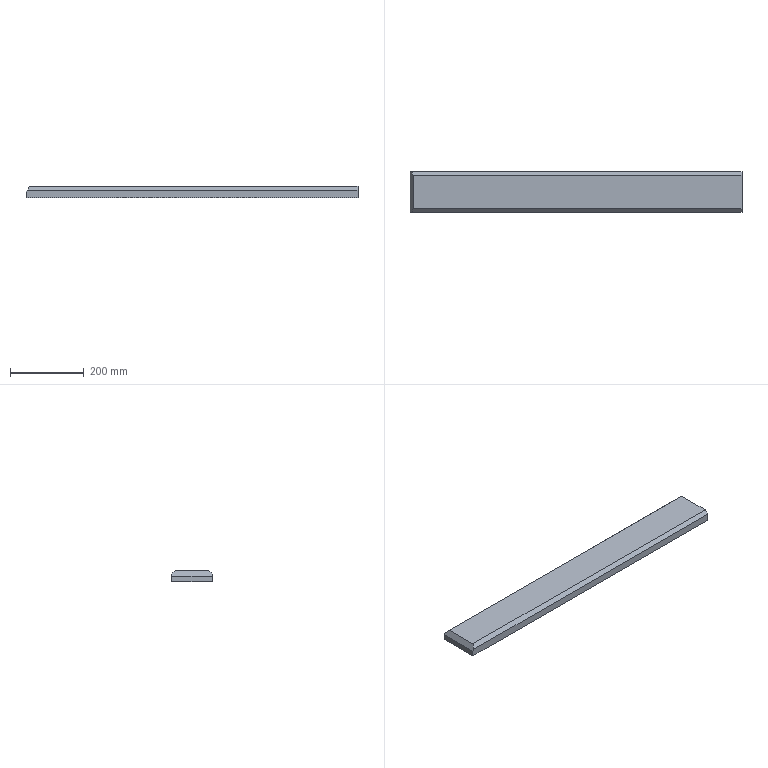Part | SolidWorks | features Chamfer 2, 3DProfileFeature 1, Extrusion 1, HoleWzd 1 | 1 solid | 13 faces | box 900 x 110 x 30 mm | volume 2865385 mm3 | plane 9 | cylinder 2 | cone 2 | commonest cylinder face diameters 14 x2
STEP:
#1=CARTESIAN_POINT('',(855.,55.,22.));
#2=VERTEX_POINT('',#1);
#3=CARTESIAN_POINT('',(855.,55.,8.));
#4=VERTEX_POINT('',#3);
#5=CARTESIAN_POINT('',(855.,55.,15.));
#6=DIRECTION('',(1.,0.,0.));
#7=DIRECTION('',(0.,0.,-1.));
#8=AXIS2_PLACEMENT_3D('',#5,#6,#7);
#9=CIRCLE('',#8,7.);
#10=EDGE_CURVE('',#2,#4,#9,.T.);
#11=ORIENTED_EDGE('',*,*,#10,.F.);
#12=CARTESIAN_POINT('',(900.,55.,22.));
#13=VERTEX_POINT('',#12);
#14=CARTESIAN_POINT('',(900.,55.,22.));
#15=DIRECTION('',(1.,0.,0.));
#16=VECTOR('',#15,1000.);
#17=LINE('',#14,#16);
#18=EDGE_CURVE('',#2,#13,#17,.T.);
#19=ORIENTED_EDGE('',*,*,#18,.T.);
#20=CARTESIAN_POINT('',(900.,55.,8.));
#21=VERTEX_POINT('',#20);
#22=CARTESIAN_POINT('',(900.,55.,15.));
#23=DIRECTION('',(1.,0.,0.));
#24=DIRECTION('',(0.,0.,-1.));
#25=AXIS2_PLACEMENT_3D('',#22,#23,#24);
#26=CIRCLE('',#25,7.);
#27=EDGE_CURVE('',#13,#21,#26,.T.);
#28=ORIENTED_EDGE('',*,*,#27,.T.);
#29=CARTESIAN_POINT('',(900.,55.,8.));
#30=DIRECTION('',(1.,0.,0.));
#31=VECTOR('',#30,1000.);
#32=LINE('',#29,#31);
#33=EDGE_CURVE('',#4,#21,#32,.T.);
#34=ORIENTED_EDGE('',*,*,#33,.F.);
#35=EDGE_LOOP('',(#11,#19,#28,#34));
#36=FACE_OUTER_BOUND('',#35,.T.);
#37=CARTESIAN_POINT('',(900.,55.,15.));
#38=DIRECTION('',(1.,0.,0.));
#39=DIRECTION('',(0.,0.,-1.));
#40=AXIS2_PLACEMENT_3D('',#37,#38,#39);
#41=CYLINDRICAL_SURFACE('',#40,7.);
#42=ADVANCED_FACE('',(#36),#41,.F.);
#43=CARTESIAN_POINT('',(850.794,55.,15.));
#44=VERTEX_POINT('',#43);
#45=CARTESIAN_POINT('',(855.,55.,8.));
#46=DIRECTION('',(0.515,0.,-0.8572));
#47=VECTOR('',#46,1000.);
#48=LINE('',#45,#47);
#49=EDGE_CURVE('',#44,#4,#48,.T.);
#50=ORIENTED_EDGE('',*,*,#49,.F.);
#51=CARTESIAN_POINT('',(855.,55.,22.));
#52=DIRECTION('',(0.515,0.,0.8572));
#53=VECTOR('',#52,1000.);
#54=LINE('',#51,#53);
#55=EDGE_CURVE('',#44,#2,#54,.T.);
#56=ORIENTED_EDGE('',*,*,#55,.T.);
#57=ORIENTED_EDGE('',*,*,#10,.T.);
#58=EDGE_LOOP('',(#50,#56,#57));
#59=FACE_OUTER_BOUND('',#58,.T.);
#60=CARTESIAN_POINT('',(855.,55.,15.));
#61=DIRECTION('',(1.,0.,0.));
#62=DIRECTION('',(0.,0.,-1.));
#63=AXIS2_PLACEMENT_3D('',#60,#61,#62);
#64=CONICAL_SURFACE('',#63,7.,1.03);
#65=ADVANCED_FACE('',(#59),#64,.F.);
#66=CARTESIAN_POINT('',(0.,0.,15.));
#67=VERTEX_POINT('',#66);
#68=CARTESIAN_POINT('',(0.,0.,0.));
#69=VERTEX_POINT('',#68);
#70=CARTESIAN_POINT('',(0.,0.,30.));
#71=DIRECTION('',(0.,0.,-1.));
#72=VECTOR('',#71,1000.);
#73=LINE('',#70,#72);
#74=EDGE_CURVE('',#67,#69,#73,.T.);
#75=ORIENTED_EDGE('',*,*,#74,.F.);
#76=CARTESIAN_POINT('',(0.,110.,15.));
#77=VERTEX_POINT('',#76);
#78=CARTESIAN_POINT('',(0.,0.,15.));
#79=DIRECTION('',(0.,1.,0.));
#80=VECTOR('',#79,1000.);
#81=LINE('',#78,#80);
#82=EDGE_CURVE('',#67,#77,#81,.T.);
#83=ORIENTED_EDGE('',*,*,#82,.T.);
#84=CARTESIAN_POINT('',(0.,110.,0.));
#85=VERTEX_POINT('',#84);
#86=CARTESIAN_POINT('',(0.,110.,30.));
#87=DIRECTION('',(0.,0.,-1.));
#88=VECTOR('',#87,1000.);
#89=LINE('',#86,#88);
#90=EDGE_CURVE('',#77,#85,#89,.T.);
#91=ORIENTED_EDGE('',*,*,#90,.T.);
#92=CARTESIAN_POINT('',(0.,0.,0.));
#93=DIRECTION('',(0.,-1.,0.));
#94=VECTOR('',#93,1000.);
#95=LINE('',#92,#94);
#96=EDGE_CURVE('',#85,#69,#95,.T.);
#97=ORIENTED_EDGE('',*,*,#96,.T.);
#98=EDGE_LOOP('',(#75,#83,#91,#97));
#99=FACE_OUTER_BOUND('',#98,.T.);
#100=CARTESIAN_POINT('',(0.,0.,30.));
#101=DIRECTION('',(1.,0.,0.));
#102=DIRECTION('',(0.,0.,-1.));
#103=AXIS2_PLACEMENT_3D('',#100,#101,#102);
#104=PLANE('',#103);
#105=ADVANCED_FACE('',(#99),#104,.F.);
#106=CARTESIAN_POINT('',(900.,0.,20.));
#107=VERTEX_POINT('',#106);
#108=CARTESIAN_POINT('',(3.333,0.,20.));
#109=VERTEX_POINT('',#108);
#110=CARTESIAN_POINT('',(0.,0.,20.));
#111=DIRECTION('',(-1.,0.,0.));
#112=VECTOR('',#111,1000.);
#113=LINE('',#110,#112);
#114=EDGE_CURVE('',#107,#109,#113,.T.);
#115=ORIENTED_EDGE('',*,*,#114,.T.);
#116=CARTESIAN_POINT('',(10.,0.,30.));
#117=DIRECTION('',(-0.5547,0.,-0.8321));
#118=VECTOR('',#117,1000.);
#119=LINE('',#116,#118);
#120=EDGE_CURVE('',#109,#67,#119,.T.);
#121=ORIENTED_EDGE('',*,*,#120,.T.);
#122=ORIENTED_EDGE('',*,*,#74,.T.);
#123=CARTESIAN_POINT('',(900.,0.,0.));
#124=VERTEX_POINT('',#123);
#125=CARTESIAN_POINT('',(0.,0.,0.));
#126=DIRECTION('',(1.,0.,0.));
#127=VECTOR('',#126,1000.);
#128=LINE('',#125,#127);
#129=EDGE_CURVE('',#69,#124,#128,.T.);
#130=ORIENTED_EDGE('',*,*,#129,.T.);
#131=CARTESIAN_POINT('',(900.,0.,30.));
#132=DIRECTION('',(0.,0.,-1.));
#133=VECTOR('',#132,1000.);
#134=LINE('',#131,#133);
#135=EDGE_CURVE('',#107,#124,#134,.T.);
#136=ORIENTED_EDGE('',*,*,#135,.F.);
#137=EDGE_LOOP('',(#115,#121,#122,#130,#136));
#138=FACE_OUTER_BOUND('',#137,.T.);
#139=CARTESIAN_POINT('',(0.,0.,30.));
#140=DIRECTION('',(0.,1.,0.));
#141=DIRECTION('',(0.,0.,1.));
#142=AXIS2_PLACEMENT_3D('',#139,#140,#141);
#143=PLANE('',#142);
#144=ADVANCED_FACE('',(#138),#143,.F.);
#145=CARTESIAN_POINT('',(900.,55.,15.));
#146=DIRECTION('',(1.,0.,0.));
#147=DIRECTION('',(0.,0.,-1.));
#148=AXIS2_PLACEMENT_3D('',#145,#146,#147);
#149=CIRCLE('',#148,7.);
#150=EDGE_CURVE('',#21,#13,#149,.T.);
#151=ORIENTED_EDGE('',*,*,#150,.F.);
#152=ORIENTED_EDGE('',*,*,#27,.F.);
#153=EDGE_LOOP('',(#151,#152));
#154=FACE_BOUND('',#153,.T.);
#155=CARTESIAN_POINT('',(900.,110.,20.));
#156=VERTEX_POINT('',#155);
#157=CARTESIAN_POINT('',(900.,110.,0.));
#158=VERTEX_POINT('',#157);
#159=CARTESIAN_POINT('',(900.,110.,30.));
#160=DIRECTION('',(0.,0.,-1.));
#161=VECTOR('',#160,1000.);
#162=LINE('',#159,#161);
#163=EDGE_CURVE('',#156,#158,#162,.T.);
#164=ORIENTED_EDGE('',*,*,#163,.F.);
#165=CARTESIAN_POINT('',(900.,100.,30.));
#166=VERTEX_POINT('',#165);
#167=CARTESIAN_POINT('',(900.,100.,30.));
#168=DIRECTION('',(0.,-0.7071,0.7071));
#169=VECTOR('',#168,1000.);
#170=LINE('',#167,#169);
#171=EDGE_CURVE('',#156,#166,#170,.T.);
#172=ORIENTED_EDGE('',*,*,#171,.T.);
#173=CARTESIAN_POINT('',(900.,10.,30.));
#174=VERTEX_POINT('',#173);
#175=CARTESIAN_POINT('',(900.,0.,30.));
#176=DIRECTION('',(0.,1.,0.));
#177=VECTOR('',#176,1000.);
#178=LINE('',#175,#177);
#179=EDGE_CURVE('',#174,#166,#178,.T.);
#180=ORIENTED_EDGE('',*,*,#179,.F.);
#181=CARTESIAN_POINT('',(900.,10.,30.));
#182=DIRECTION('',(0.,-0.7071,-0.7071));
#183=VECTOR('',#182,1000.);
#184=LINE('',#181,#183);
#185=EDGE_CURVE('',#174,#107,#184,.T.);
#186=ORIENTED_EDGE('',*,*,#185,.T.);
#187=ORIENTED_EDGE('',*,*,#135,.T.);
#188=CARTESIAN_POINT('',(900.,0.,0.));
#189=DIRECTION('',(0.,1.,0.));
#190=VECTOR('',#189,1000.);
#191=LINE('',#188,#190);
#192=EDGE_CURVE('',#124,#158,#191,.T.);
#193=ORIENTED_EDGE('',*,*,#192,.T.);
#194=EDGE_LOOP('',(#164,#172,#180,#186,#187,#193));
#195=FACE_OUTER_BOUND('',#194,.T.);
#196=CARTESIAN_POINT('',(900.,0.,30.));
#197=DIRECTION('',(-1.,0.,0.));
#198=DIRECTION('',(0.,0.,1.));
#199=AXIS2_PLACEMENT_3D('',#196,#197,#198);
#200=PLANE('',#199);
#201=ADVANCED_FACE('',(#154,#195),#200,.F.);
#202=ORIENTED_EDGE('',*,*,#90,.F.);
#203=CARTESIAN_POINT('',(3.333,110.,20.));
#204=VERTEX_POINT('',#203);
#205=CARTESIAN_POINT('',(10.,110.,30.));
#206=DIRECTION('',(0.5547,0.,0.8321));
#207=VECTOR('',#206,1000.);
#208=LINE('',#205,#207);
#209=EDGE_CURVE('',#77,#204,#208,.T.);
#210=ORIENTED_EDGE('',*,*,#209,.T.);
#211=CARTESIAN_POINT('',(0.,110.,20.));
#212=DIRECTION('',(1.,0.,0.));
#213=VECTOR('',#212,1000.);
#214=LINE('',#211,#213);
#215=EDGE_CURVE('',#204,#156,#214,.T.);
#216=ORIENTED_EDGE('',*,*,#215,.T.);
#217=ORIENTED_EDGE('',*,*,#163,.T.);
#218=CARTESIAN_POINT('',(0.,110.,0.));
#219=DIRECTION('',(-1.,0.,0.));
#220=VECTOR('',#219,1000.);
#221=LINE('',#218,#220);
#222=EDGE_CURVE('',#158,#85,#221,.T.);
#223=ORIENTED_EDGE('',*,*,#222,.T.);
#224=EDGE_LOOP('',(#202,#210,#216,#217,#223));
#225=FACE_OUTER_BOUND('',#224,.T.);
#226=CARTESIAN_POINT('',(0.,110.,30.));
#227=DIRECTION('',(0.,-1.,0.));
#228=DIRECTION('',(0.,0.,-1.));
#229=AXIS2_PLACEMENT_3D('',#226,#227,#228);
#230=PLANE('',#229);
#231=ADVANCED_FACE('',(#225),#230,.F.);
#232=CARTESIAN_POINT('',(10.,100.,30.));
#233=VERTEX_POINT('',#232);
#234=CARTESIAN_POINT('',(0.,100.,30.));
#235=DIRECTION('',(-1.,0.,0.));
#236=VECTOR('',#235,1000.);
#237=LINE('',#234,#236);
#238=EDGE_CURVE('',#166,#233,#237,.T.);
#239=ORIENTED_EDGE('',*,*,#238,.T.);
#240=CARTESIAN_POINT('',(10.,10.,30.));
#241=VERTEX_POINT('',#240);
#242=CARTESIAN_POINT('',(10.,0.,30.));
#243=DIRECTION('',(0.,-1.,0.));
#244=VECTOR('',#243,1000.);
#245=LINE('',#242,#244);
#246=EDGE_CURVE('',#233,#241,#245,.T.);
#247=ORIENTED_EDGE('',*,*,#246,.T.);
#248=CARTESIAN_POINT('',(0.,10.,30.));
#249=DIRECTION('',(1.,0.,0.));
#250=VECTOR('',#249,1000.);
#251=LINE('',#248,#250);
#252=EDGE_CURVE('',#241,#174,#251,.T.);
#253=ORIENTED_EDGE('',*,*,#252,.T.);
#254=ORIENTED_EDGE('',*,*,#179,.T.);
#255=EDGE_LOOP('',(#239,#247,#253,#254));
#256=FACE_OUTER_BOUND('',#255,.T.);
#257=CARTESIAN_POINT('',(0.,0.,30.));
#258=DIRECTION('',(0.,0.,-1.));
#259=DIRECTION('',(-1.,0.,0.));
#260=AXIS2_PLACEMENT_3D('',#257,#258,#259);
#261=PLANE('',#260);
#262=ADVANCED_FACE('',(#256),#261,.F.);
#263=ORIENTED_EDGE('',*,*,#96,.F.);
#264=ORIENTED_EDGE('',*,*,#222,.F.);
#265=ORIENTED_EDGE('',*,*,#192,.F.);
#266=ORIENTED_EDGE('',*,*,#129,.F.);
#267=EDGE_LOOP('',(#263,#264,#265,#266));
#268=FACE_OUTER_BOUND('',#267,.T.);
#269=CARTESIAN_POINT('',(0.,0.,0.));
#270=DIRECTION('',(0.,0.,-1.));
#271=DIRECTION('',(-1.,0.,0.));
#272=AXIS2_PLACEMENT_3D('',#269,#270,#271);
#273=PLANE('',#272);
#274=ADVANCED_FACE('',(#268),#273,.T.);
#275=ORIENTED_EDGE('',*,*,#215,.F.);
#276=CARTESIAN_POINT('',(8.182,102.727,27.273));
#277=DIRECTION('',(0.4264,-0.6396,0.6396));
#278=VECTOR('',#277,1000.);
#279=LINE('',#276,#278);
#280=EDGE_CURVE('',#204,#233,#279,.T.);
#281=ORIENTED_EDGE('',*,*,#280,.T.);
#282=ORIENTED_EDGE('',*,*,#238,.F.);
#283=ORIENTED_EDGE('',*,*,#171,.F.);
#284=EDGE_LOOP('',(#275,#281,#282,#283));
#285=FACE_OUTER_BOUND('',#284,.T.);
#286=CARTESIAN_POINT('',(0.,100.,30.));
#287=DIRECTION('',(0.,-0.7071,-0.7071));
#288=DIRECTION('',(-1.,0.,0.));
#289=AXIS2_PLACEMENT_3D('',#286,#287,#288);
#290=PLANE('',#289);
#291=ADVANCED_FACE('',(#285),#290,.F.);
#292=ORIENTED_EDGE('',*,*,#252,.F.);
#293=CARTESIAN_POINT('',(8.182,7.273,27.273));
#294=DIRECTION('',(-0.4264,-0.6396,-0.6396));
#295=VECTOR('',#294,1000.);
#296=LINE('',#293,#295);
#297=EDGE_CURVE('',#241,#109,#296,.T.);
#298=ORIENTED_EDGE('',*,*,#297,.T.);
#299=ORIENTED_EDGE('',*,*,#114,.F.);
#300=ORIENTED_EDGE('',*,*,#185,.F.);
#301=EDGE_LOOP('',(#292,#298,#299,#300));
#302=FACE_OUTER_BOUND('',#301,.T.);
#303=CARTESIAN_POINT('',(0.,10.,30.));
#304=DIRECTION('',(0.,0.7071,-0.7071));
#305=DIRECTION('',(1.,0.,0.));
#306=AXIS2_PLACEMENT_3D('',#303,#304,#305);
#307=PLANE('',#306);
#308=ADVANCED_FACE('',(#302),#307,.F.);
#309=ORIENTED_EDGE('',*,*,#209,.F.);
#310=ORIENTED_EDGE('',*,*,#82,.F.);
#311=ORIENTED_EDGE('',*,*,#120,.F.);
#312=ORIENTED_EDGE('',*,*,#297,.F.);
#313=ORIENTED_EDGE('',*,*,#246,.F.);
#314=ORIENTED_EDGE('',*,*,#280,.F.);
#315=EDGE_LOOP('',(#309,#310,#311,#312,#313,#314));
#316=FACE_OUTER_BOUND('',#315,.T.);
#317=CARTESIAN_POINT('',(10.,0.,30.));
#318=DIRECTION('',(0.8321,0.,-0.5547));
#319=DIRECTION('',(0.,-1.,0.));
#320=AXIS2_PLACEMENT_3D('',#317,#318,#319);
#321=PLANE('',#320);
#322=ADVANCED_FACE('',(#316),#321,.F.);
#323=ORIENTED_EDGE('',*,*,#55,.F.);
#324=ORIENTED_EDGE('',*,*,#49,.T.);
#325=CARTESIAN_POINT('',(855.,55.,15.));
#326=DIRECTION('',(1.,0.,0.));
#327=DIRECTION('',(0.,0.,-1.));
#328=AXIS2_PLACEMENT_3D('',#325,#326,#327);
#329=CIRCLE('',#328,7.);
#330=EDGE_CURVE('',#4,#2,#329,.T.);
#331=ORIENTED_EDGE('',*,*,#330,.T.);
#332=EDGE_LOOP('',(#323,#324,#331));
#333=FACE_OUTER_BOUND('',#332,.T.);
#334=CARTESIAN_POINT('',(855.,55.,15.));
#335=DIRECTION('',(1.,0.,0.));
#336=DIRECTION('',(0.,0.,-1.));
#337=AXIS2_PLACEMENT_3D('',#334,#335,#336);
#338=CONICAL_SURFACE('',#337,7.,1.03);
#339=ADVANCED_FACE('',(#333),#338,.F.);
#340=ORIENTED_EDGE('',*,*,#18,.F.);
#341=ORIENTED_EDGE('',*,*,#330,.F.);
#342=ORIENTED_EDGE('',*,*,#33,.T.);
#343=ORIENTED_EDGE('',*,*,#150,.T.);
#344=EDGE_LOOP('',(#340,#341,#342,#343));
#345=FACE_OUTER_BOUND('',#344,.T.);
#346=CARTESIAN_POINT('',(900.,55.,15.));
#347=DIRECTION('',(1.,0.,0.));
#348=DIRECTION('',(0.,0.,-1.));
#349=AXIS2_PLACEMENT_3D('',#346,#347,#348);
#350=CYLINDRICAL_SURFACE('',#349,7.);
#351=ADVANCED_FACE('',(#345),#350,.F.);
#352=CLOSED_SHELL('',(#42,#65,#105,#144,#201,#231,#262,#274,#291,#308,#322,#339,#351));
#353=MANIFOLD_SOLID_BREP('',#352);
#354=CARTESIAN_POINT('',(0.,0.,0.));
#355=DIRECTION('',(0.,0.,1.));
#356=DIRECTION('',(1.,0.,0.));
#357=AXIS2_PLACEMENT_3D('',#354,#355,#356);
#358=(LENGTH_UNIT()NAMED_UNIT(*)SI_UNIT(.MILLI.,.METRE.));
#359=UNCERTAINTY_MEASURE_WITH_UNIT(LENGTH_MEASURE(0.00001),#358,'','');
#360=(NAMED_UNIT(*)PLANE_ANGLE_UNIT()SI_UNIT($,.RADIAN.));
#361=(NAMED_UNIT(*)SI_UNIT($,.STERADIAN.)SOLID_ANGLE_UNIT());
#362=(GEOMETRIC_REPRESENTATION_CONTEXT(3)GLOBAL_UNCERTAINTY_ASSIGNED_CONTEXT((#359))GLOBAL_UNIT_ASSIGNED_CONTEXT((#358,#360,#361))REPRESENTATION_CONTEXT('',''));
#363=ADVANCED_BREP_SHAPE_REPRESENTATION('',(#353,#357),#362);